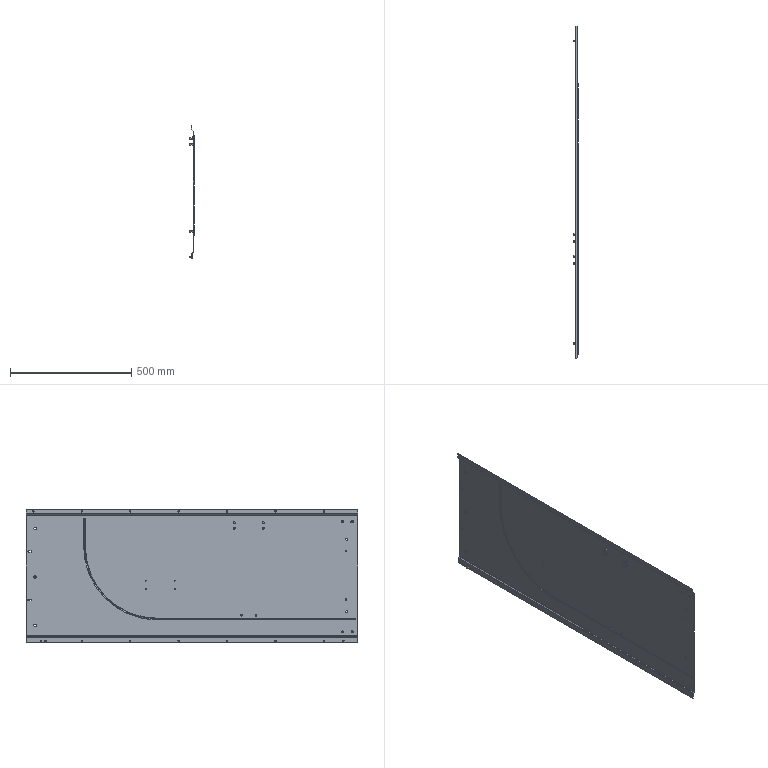Part | STEP file | 64741551 | 1 solid | 201 faces | box 17.8 x 1370 x 552 mm | volume 1150398 mm3 | cylinder 114 | plane 57 | torus 26 | sphere 4 | commonest cylinder face diameters 6 x37 5 x20 4 x14 7.8 x12 8 x12 10 x6